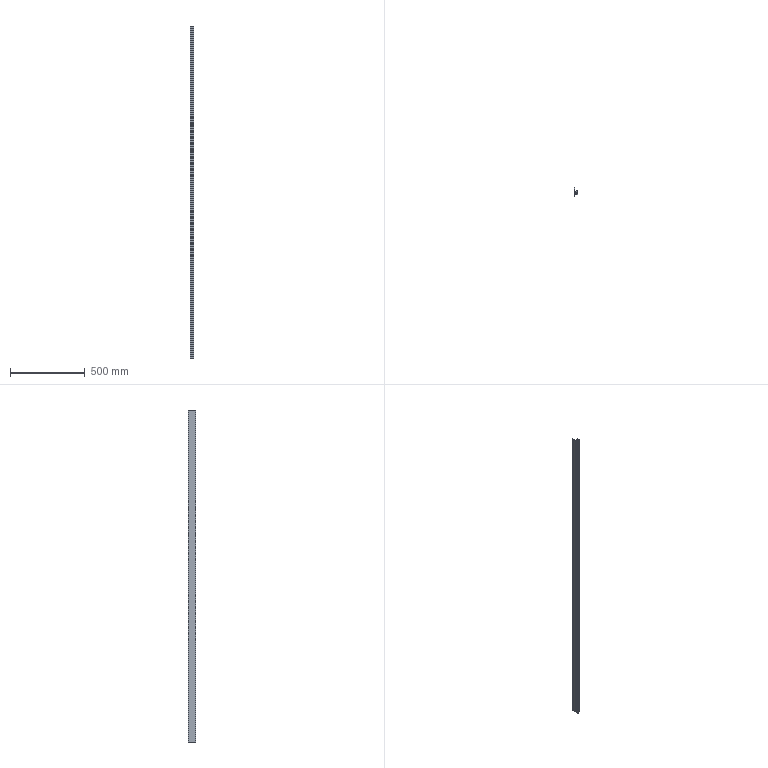Part | SolidWorks | features Extrusion 1 | 1 solid | 43 faces | box 25 x 50 x 2216 mm | volume 690351 mm3 | plane 35 | cylinder 8 | commonest cylinder face diameters 0.6 x8
STEP:
#1=CARTESIAN_POINT('',(1.5,0.,1108.));
#2=VERTEX_POINT('',#1);
#3=CARTESIAN_POINT('',(1.5,10.,1108.));
#4=VERTEX_POINT('',#3);
#5=CARTESIAN_POINT('',(1.5,0.,1108.));
#6=DIRECTION('',(0.,1.,0.));
#7=VECTOR('',#6,1000.);
#8=LINE('',#5,#7);
#9=EDGE_CURVE('',#2,#4,#8,.T.);
#10=ORIENTED_EDGE('',*,*,#9,.T.);
#11=CARTESIAN_POINT('',(4.,10.,1108.));
#12=VERTEX_POINT('',#11);
#13=CARTESIAN_POINT('',(1.5,10.,1108.));
#14=DIRECTION('',(1.,0.,0.));
#15=VECTOR('',#14,1000.);
#16=LINE('',#13,#15);
#17=EDGE_CURVE('',#4,#12,#16,.T.);
#18=ORIENTED_EDGE('',*,*,#17,.T.);
#19=CARTESIAN_POINT('',(4.,10.5,1108.));
#20=VERTEX_POINT('',#19);
#21=CARTESIAN_POINT('',(4.,10.,1108.));
#22=DIRECTION('',(0.,1.,0.));
#23=VECTOR('',#22,1000.);
#24=LINE('',#21,#23);
#25=EDGE_CURVE('',#12,#20,#24,.T.);
#26=ORIENTED_EDGE('',*,*,#25,.T.);
#27=CARTESIAN_POINT('',(8.9,10.5,1108.));
#28=VERTEX_POINT('',#27);
#29=CARTESIAN_POINT('',(4.,10.5,1108.));
#30=DIRECTION('',(1.,0.,0.));
#31=VECTOR('',#30,1000.);
#32=LINE('',#29,#31);
#33=EDGE_CURVE('',#20,#28,#32,.T.);
#34=ORIENTED_EDGE('',*,*,#33,.T.);
#35=CARTESIAN_POINT('',(8.9,12.2,1108.));
#36=VERTEX_POINT('',#35);
#37=CARTESIAN_POINT('',(8.9,10.5,1108.));
#38=DIRECTION('',(0.,1.,0.));
#39=VECTOR('',#38,1000.);
#40=LINE('',#37,#39);
#41=EDGE_CURVE('',#28,#36,#40,.T.);
#42=ORIENTED_EDGE('',*,*,#41,.T.);
#43=CARTESIAN_POINT('',(8.6,12.5,1108.));
#44=VERTEX_POINT('',#43);
#45=CARTESIAN_POINT('',(8.6,12.2,1108.));
#46=DIRECTION('',(0.,0.,1.));
#47=DIRECTION('',(1.,0.,0.));
#48=AXIS2_PLACEMENT_3D('',#45,#46,#47);
#49=CIRCLE('',#48,0.3);
#50=EDGE_CURVE('',#36,#44,#49,.T.);
#51=ORIENTED_EDGE('',*,*,#50,.T.);
#52=CARTESIAN_POINT('',(5.05,12.5,1108.));
#53=VERTEX_POINT('',#52);
#54=CARTESIAN_POINT('',(8.6,12.5,1108.));
#55=DIRECTION('',(-1.,0.,0.));
#56=VECTOR('',#55,1000.);
#57=LINE('',#54,#56);
#58=EDGE_CURVE('',#44,#53,#57,.T.);
#59=ORIENTED_EDGE('',*,*,#58,.T.);
#60=CARTESIAN_POINT('',(4.75,12.8,1108.));
#61=VERTEX_POINT('',#60);
#62=CARTESIAN_POINT('',(5.05,12.8,1108.));
#63=DIRECTION('',(0.,0.,-1.));
#64=DIRECTION('',(1.,0.,0.));
#65=AXIS2_PLACEMENT_3D('',#62,#63,#64);
#66=CIRCLE('',#65,0.3);
#67=EDGE_CURVE('',#53,#61,#66,.T.);
#68=ORIENTED_EDGE('',*,*,#67,.T.);
#69=CARTESIAN_POINT('',(4.75,16.153,1108.));
#70=VERTEX_POINT('',#69);
#71=CARTESIAN_POINT('',(4.75,12.8,1108.));
#72=DIRECTION('',(0.,1.,0.));
#73=VECTOR('',#72,1000.);
#74=LINE('',#71,#73);
#75=EDGE_CURVE('',#61,#70,#74,.T.);
#76=ORIENTED_EDGE('',*,*,#75,.T.);
#77=CARTESIAN_POINT('',(4.838,16.365,1108.));
#78=VERTEX_POINT('',#77);
#79=CARTESIAN_POINT('',(5.05,16.153,1108.));
#80=DIRECTION('',(0.,0.,-1.));
#81=DIRECTION('',(1.,0.,0.));
#82=AXIS2_PLACEMENT_3D('',#79,#80,#81);
#83=CIRCLE('',#82,0.3);
#84=EDGE_CURVE('',#70,#78,#83,.T.);
#85=ORIENTED_EDGE('',*,*,#84,.T.);
#86=CARTESIAN_POINT('',(8.785,20.312,1108.));
#87=VERTEX_POINT('',#86);
#88=CARTESIAN_POINT('',(4.838,16.365,1108.));
#89=DIRECTION('',(0.7071,0.7071,0.));
#90=VECTOR('',#89,1000.);
#91=LINE('',#88,#90);
#92=EDGE_CURVE('',#78,#87,#91,.T.);
#93=ORIENTED_EDGE('',*,*,#92,.T.);
#94=CARTESIAN_POINT('',(8.997,20.4,1108.));
#95=VERTEX_POINT('',#94);
#96=CARTESIAN_POINT('',(8.997,20.1,1108.));
#97=DIRECTION('',(0.,0.,-1.));
#98=DIRECTION('',(1.,0.,0.));
#99=AXIS2_PLACEMENT_3D('',#96,#97,#98);
#100=CIRCLE('',#99,0.3);
#101=EDGE_CURVE('',#87,#95,#100,.T.);
#102=ORIENTED_EDGE('',*,*,#101,.T.);
#103=CARTESIAN_POINT('',(17.003,20.4,1108.));
#104=VERTEX_POINT('',#103);
#105=CARTESIAN_POINT('',(8.997,20.4,1108.));
#106=DIRECTION('',(1.,0.,0.));
#107=VECTOR('',#106,1000.);
#108=LINE('',#105,#107);
#109=EDGE_CURVE('',#95,#104,#108,.T.);
#110=ORIENTED_EDGE('',*,*,#109,.T.);
#111=CARTESIAN_POINT('',(17.215,20.312,1108.));
#112=VERTEX_POINT('',#111);
#113=CARTESIAN_POINT('',(17.003,20.1,1108.));
#114=DIRECTION('',(0.,0.,-1.));
#115=DIRECTION('',(1.,0.,0.));
#116=AXIS2_PLACEMENT_3D('',#113,#114,#115);
#117=CIRCLE('',#116,0.3);
#118=EDGE_CURVE('',#104,#112,#117,.T.);
#119=ORIENTED_EDGE('',*,*,#118,.T.);
#120=CARTESIAN_POINT('',(21.162,16.365,1108.));
#121=VERTEX_POINT('',#120);
#122=CARTESIAN_POINT('',(17.215,20.312,1108.));
#123=DIRECTION('',(0.7071,-0.7071,0.));
#124=VECTOR('',#123,1000.);
#125=LINE('',#122,#124);
#126=EDGE_CURVE('',#112,#121,#125,.T.);
#127=ORIENTED_EDGE('',*,*,#126,.T.);
#128=CARTESIAN_POINT('',(21.25,16.153,1108.));
#129=VERTEX_POINT('',#128);
#130=CARTESIAN_POINT('',(20.95,16.153,1108.));
#131=DIRECTION('',(0.,0.,-1.));
#132=DIRECTION('',(1.,0.,0.));
#133=AXIS2_PLACEMENT_3D('',#130,#131,#132);
#134=CIRCLE('',#133,0.3);
#135=EDGE_CURVE('',#121,#129,#134,.T.);
#136=ORIENTED_EDGE('',*,*,#135,.T.);
#137=CARTESIAN_POINT('',(21.25,12.8,1108.));
#138=VERTEX_POINT('',#137);
#139=CARTESIAN_POINT('',(21.25,16.153,1108.));
#140=DIRECTION('',(0.,-1.,0.));
#141=VECTOR('',#140,1000.);
#142=LINE('',#139,#141);
#143=EDGE_CURVE('',#129,#138,#142,.T.);
#144=ORIENTED_EDGE('',*,*,#143,.T.);
#145=CARTESIAN_POINT('',(20.95,12.5,1108.));
#146=VERTEX_POINT('',#145);
#147=CARTESIAN_POINT('',(20.95,12.8,1108.));
#148=DIRECTION('',(0.,0.,-1.));
#149=DIRECTION('',(1.,0.,0.));
#150=AXIS2_PLACEMENT_3D('',#147,#148,#149);
#151=CIRCLE('',#150,0.3);
#152=EDGE_CURVE('',#138,#146,#151,.T.);
#153=ORIENTED_EDGE('',*,*,#152,.T.);
#154=CARTESIAN_POINT('',(17.4,12.5,1108.));
#155=VERTEX_POINT('',#154);
#156=CARTESIAN_POINT('',(20.95,12.5,1108.));
#157=DIRECTION('',(-1.,0.,0.));
#158=VECTOR('',#157,1000.);
#159=LINE('',#156,#158);
#160=EDGE_CURVE('',#146,#155,#159,.T.);
#161=ORIENTED_EDGE('',*,*,#160,.T.);
#162=CARTESIAN_POINT('',(17.1,12.2,1108.));
#163=VERTEX_POINT('',#162);
#164=CARTESIAN_POINT('',(17.4,12.2,1108.));
#165=DIRECTION('',(0.,0.,1.));
#166=DIRECTION('',(1.,0.,0.));
#167=AXIS2_PLACEMENT_3D('',#164,#165,#166);
#168=CIRCLE('',#167,0.3);
#169=EDGE_CURVE('',#155,#163,#168,.T.);
#170=ORIENTED_EDGE('',*,*,#169,.T.);
#171=CARTESIAN_POINT('',(17.1,10.5,1108.));
#172=VERTEX_POINT('',#171);
#173=CARTESIAN_POINT('',(17.1,12.2,1108.));
#174=DIRECTION('',(0.,-1.,0.));
#175=VECTOR('',#174,1000.);
#176=LINE('',#173,#175);
#177=EDGE_CURVE('',#163,#172,#176,.T.);
#178=ORIENTED_EDGE('',*,*,#177,.T.);
#179=CARTESIAN_POINT('',(22.,10.5,1108.));
#180=VERTEX_POINT('',#179);
#181=CARTESIAN_POINT('',(17.1,10.5,1108.));
#182=DIRECTION('',(1.,0.,0.));
#183=VECTOR('',#182,1000.);
#184=LINE('',#181,#183);
#185=EDGE_CURVE('',#172,#180,#184,.T.);
#186=ORIENTED_EDGE('',*,*,#185,.T.);
#187=CARTESIAN_POINT('',(22.,10.,1108.));
#188=VERTEX_POINT('',#187);
#189=CARTESIAN_POINT('',(22.,10.5,1108.));
#190=DIRECTION('',(0.,-1.,0.));
#191=VECTOR('',#190,1000.);
#192=LINE('',#189,#191);
#193=EDGE_CURVE('',#180,#188,#192,.T.);
#194=ORIENTED_EDGE('',*,*,#193,.T.);
#195=CARTESIAN_POINT('',(25.,10.,1108.));
#196=VERTEX_POINT('',#195);
#197=CARTESIAN_POINT('',(22.,10.,1108.));
#198=DIRECTION('',(1.,0.,0.));
#199=VECTOR('',#198,1000.);
#200=LINE('',#197,#199);
#201=EDGE_CURVE('',#188,#196,#200,.T.);
#202=ORIENTED_EDGE('',*,*,#201,.T.);
#203=CARTESIAN_POINT('',(25.,15.,1108.));
#204=VERTEX_POINT('',#203);
#205=CARTESIAN_POINT('',(25.,10.,1108.));
#206=DIRECTION('',(0.,1.,0.));
#207=VECTOR('',#206,1000.);
#208=LINE('',#205,#207);
#209=EDGE_CURVE('',#196,#204,#208,.T.);
#210=ORIENTED_EDGE('',*,*,#209,.T.);
#211=CARTESIAN_POINT('',(23.,15.,1108.));
#212=VERTEX_POINT('',#211);
#213=CARTESIAN_POINT('',(25.,15.,1108.));
#214=DIRECTION('',(-1.,0.,0.));
#215=VECTOR('',#214,1000.);
#216=LINE('',#213,#215);
#217=EDGE_CURVE('',#204,#212,#216,.T.);
#218=ORIENTED_EDGE('',*,*,#217,.T.);
#219=CARTESIAN_POINT('',(23.,29.246,1108.));
#220=VERTEX_POINT('',#219);
#221=CARTESIAN_POINT('',(23.,15.,1108.));
#222=DIRECTION('',(0.,1.,0.));
#223=VECTOR('',#222,1000.);
#224=LINE('',#221,#223);
#225=EDGE_CURVE('',#212,#220,#224,.T.);
#226=ORIENTED_EDGE('',*,*,#225,.T.);
#227=CARTESIAN_POINT('',(22.25,29.996,1108.));
#228=VERTEX_POINT('',#227);
#229=CARTESIAN_POINT('',(23.,29.246,1108.));
#230=DIRECTION('',(-0.7071,0.7071,0.));
#231=VECTOR('',#230,1000.);
#232=LINE('',#229,#231);
#233=EDGE_CURVE('',#220,#228,#232,.T.);
#234=ORIENTED_EDGE('',*,*,#233,.T.);
#235=CARTESIAN_POINT('',(4.,30.,1108.));
#236=VERTEX_POINT('',#235);
#237=CARTESIAN_POINT('',(22.25,29.996,1108.));
#238=DIRECTION('',(-1.,0.0002341,0.));
#239=VECTOR('',#238,1000.);
#240=LINE('',#237,#239);
#241=EDGE_CURVE('',#228,#236,#240,.T.);
#242=ORIENTED_EDGE('',*,*,#241,.T.);
#243=CARTESIAN_POINT('',(4.,34.998,1108.));
#244=VERTEX_POINT('',#243);
#245=CARTESIAN_POINT('',(4.,30.,1108.));
#246=DIRECTION('',(0.,1.,0.));
#247=VECTOR('',#246,1000.);
#248=LINE('',#245,#247);
#249=EDGE_CURVE('',#236,#244,#248,.T.);
#250=ORIENTED_EDGE('',*,*,#249,.T.);
#251=CARTESIAN_POINT('',(3.,34.998,1108.));
#252=VERTEX_POINT('',#251);
#253=CARTESIAN_POINT('',(4.,34.998,1108.));
#254=DIRECTION('',(-1.,0.,0.));
#255=VECTOR('',#254,1000.);
#256=LINE('',#253,#255);
#257=EDGE_CURVE('',#244,#252,#256,.T.);
#258=ORIENTED_EDGE('',*,*,#257,.T.);
#259=CARTESIAN_POINT('',(3.,43.,1108.));
#260=VERTEX_POINT('',#259);
#261=CARTESIAN_POINT('',(3.,34.998,1108.));
#262=DIRECTION('',(0.,1.,0.));
#263=VECTOR('',#262,1000.);
#264=LINE('',#261,#263);
#265=EDGE_CURVE('',#252,#260,#264,.T.);
#266=ORIENTED_EDGE('',*,*,#265,.T.);
#267=CARTESIAN_POINT('',(4.,43.,1108.));
#268=VERTEX_POINT('',#267);
#269=CARTESIAN_POINT('',(3.,43.,1108.));
#270=DIRECTION('',(1.,0.,0.));
#271=VECTOR('',#270,1000.);
#272=LINE('',#269,#271);
#273=EDGE_CURVE('',#260,#268,#272,.T.);
#274=ORIENTED_EDGE('',*,*,#273,.T.);
#275=CARTESIAN_POINT('',(4.,50.,1108.));
#276=VERTEX_POINT('',#275);
#277=CARTESIAN_POINT('',(4.,43.,1108.));
#278=DIRECTION('',(0.,1.,0.));
#279=VECTOR('',#278,1000.);
#280=LINE('',#277,#279);
#281=EDGE_CURVE('',#268,#276,#280,.T.);
#282=ORIENTED_EDGE('',*,*,#281,.T.);
#283=CARTESIAN_POINT('',(0.,50.,1108.));
#284=VERTEX_POINT('',#283);
#285=CARTESIAN_POINT('',(4.,50.,1108.));
#286=DIRECTION('',(-1.,0.,0.));
#287=VECTOR('',#286,1000.);
#288=LINE('',#285,#287);
#289=EDGE_CURVE('',#276,#284,#288,.T.);
#290=ORIENTED_EDGE('',*,*,#289,.T.);
#291=CARTESIAN_POINT('',(0.,0.,1108.));
#292=VERTEX_POINT('',#291);
#293=CARTESIAN_POINT('',(0.,50.,1108.));
#294=DIRECTION('',(0.,-1.,0.));
#295=VECTOR('',#294,1000.);
#296=LINE('',#293,#295);
#297=EDGE_CURVE('',#284,#292,#296,.T.);
#298=ORIENTED_EDGE('',*,*,#297,.T.);
#299=CARTESIAN_POINT('',(0.,0.,1108.));
#300=DIRECTION('',(1.,0.,0.));
#301=VECTOR('',#300,1000.);
#302=LINE('',#299,#301);
#303=EDGE_CURVE('',#292,#2,#302,.T.);
#304=ORIENTED_EDGE('',*,*,#303,.T.);
#305=EDGE_LOOP('',(#10,#18,#26,#34,#42,#51,#59,#68,#76,#85,#93,#102,#110,#119,#127,#136,#144,#153,#161,#170,#178,#186,#194,#202,#210,#218,#226,#234,#242,#250,#258,#266,#274,#282,#290,#298,#304));
#306=FACE_OUTER_BOUND('',#305,.T.);
#307=CARTESIAN_POINT('',(21.,28.,1108.));
#308=VERTEX_POINT('',#307);
#309=CARTESIAN_POINT('',(2.,28.,1108.));
#310=VERTEX_POINT('',#309);
#311=CARTESIAN_POINT('',(2.,28.,1108.));
#312=DIRECTION('',(-1.,0.,0.));
#313=VECTOR('',#312,1000.);
#314=LINE('',#311,#313);
#315=EDGE_CURVE('',#308,#310,#314,.T.);
#316=ORIENTED_EDGE('',*,*,#315,.F.);
#317=CARTESIAN_POINT('',(21.,22.4,1108.));
#318=VERTEX_POINT('',#317);
#319=CARTESIAN_POINT('',(21.,28.,1108.));
#320=DIRECTION('',(0.,1.,0.));
#321=VECTOR('',#320,1000.);
#322=LINE('',#319,#321);
#323=EDGE_CURVE('',#318,#308,#322,.T.);
#324=ORIENTED_EDGE('',*,*,#323,.F.);
#325=CARTESIAN_POINT('',(2.,22.4,1108.));
#326=VERTEX_POINT('',#325);
#327=CARTESIAN_POINT('',(21.,22.4,1108.));
#328=DIRECTION('',(1.,0.,0.));
#329=VECTOR('',#328,1000.);
#330=LINE('',#327,#329);
#331=EDGE_CURVE('',#326,#318,#330,.T.);
#332=ORIENTED_EDGE('',*,*,#331,.F.);
#333=CARTESIAN_POINT('',(2.,22.4,1108.));
#334=DIRECTION('',(0.,-1.,0.));
#335=VECTOR('',#334,1000.);
#336=LINE('',#333,#335);
#337=EDGE_CURVE('',#310,#326,#336,.T.);
#338=ORIENTED_EDGE('',*,*,#337,.F.);
#339=EDGE_LOOP('',(#316,#324,#332,#338));
#340=FACE_BOUND('',#339,.T.);
#341=CARTESIAN_POINT('',(8.6,12.2,1108.));
#342=DIRECTION('',(0.,0.,1.));
#343=DIRECTION('',(1.,0.,0.));
#344=AXIS2_PLACEMENT_3D('',#341,#342,#343);
#345=PLANE('',#344);
#346=ADVANCED_FACE('',(#306,#340),#345,.T.);
#347=CARTESIAN_POINT('',(1.5,0.,-1108.));
#348=VERTEX_POINT('',#347);
#349=CARTESIAN_POINT('',(1.5,10.,-1108.));
#350=VERTEX_POINT('',#349);
#351=CARTESIAN_POINT('',(1.5,0.,-1108.));
#352=DIRECTION('',(0.,1.,0.));
#353=VECTOR('',#352,1000.);
#354=LINE('',#351,#353);
#355=EDGE_CURVE('',#348,#350,#354,.T.);
#356=ORIENTED_EDGE('',*,*,#355,.F.);
#357=CARTESIAN_POINT('',(0.,0.,-1108.));
#358=VERTEX_POINT('',#357);
#359=CARTESIAN_POINT('',(0.,0.,-1108.));
#360=DIRECTION('',(1.,0.,0.));
#361=VECTOR('',#360,1000.);
#362=LINE('',#359,#361);
#363=EDGE_CURVE('',#358,#348,#362,.T.);
#364=ORIENTED_EDGE('',*,*,#363,.F.);
#365=CARTESIAN_POINT('',(0.,50.,-1108.));
#366=VERTEX_POINT('',#365);
#367=CARTESIAN_POINT('',(0.,50.,-1108.));
#368=DIRECTION('',(0.,-1.,0.));
#369=VECTOR('',#368,1000.);
#370=LINE('',#367,#369);
#371=EDGE_CURVE('',#366,#358,#370,.T.);
#372=ORIENTED_EDGE('',*,*,#371,.F.);
#373=CARTESIAN_POINT('',(4.,50.,-1108.));
#374=VERTEX_POINT('',#373);
#375=CARTESIAN_POINT('',(4.,50.,-1108.));
#376=DIRECTION('',(-1.,0.,0.));
#377=VECTOR('',#376,1000.);
#378=LINE('',#375,#377);
#379=EDGE_CURVE('',#374,#366,#378,.T.);
#380=ORIENTED_EDGE('',*,*,#379,.F.);
#381=CARTESIAN_POINT('',(4.,43.,-1108.));
#382=VERTEX_POINT('',#381);
#383=CARTESIAN_POINT('',(4.,43.,-1108.));
#384=DIRECTION('',(0.,1.,0.));
#385=VECTOR('',#384,1000.);
#386=LINE('',#383,#385);
#387=EDGE_CURVE('',#382,#374,#386,.T.);
#388=ORIENTED_EDGE('',*,*,#387,.F.);
#389=CARTESIAN_POINT('',(3.,43.,-1108.));
#390=VERTEX_POINT('',#389);
#391=CARTESIAN_POINT('',(3.,43.,-1108.));
#392=DIRECTION('',(1.,0.,0.));
#393=VECTOR('',#392,1000.);
#394=LINE('',#391,#393);
#395=EDGE_CURVE('',#390,#382,#394,.T.);
#396=ORIENTED_EDGE('',*,*,#395,.F.);
#397=CARTESIAN_POINT('',(3.,34.998,-1108.));
#398=VERTEX_POINT('',#397);
#399=CARTESIAN_POINT('',(3.,34.998,-1108.));
#400=DIRECTION('',(0.,1.,0.));
#401=VECTOR('',#400,1000.);
#402=LINE('',#399,#401);
#403=EDGE_CURVE('',#398,#390,#402,.T.);
#404=ORIENTED_EDGE('',*,*,#403,.F.);
#405=CARTESIAN_POINT('',(4.,34.998,-1108.));
#406=VERTEX_POINT('',#405);
#407=CARTESIAN_POINT('',(4.,34.998,-1108.));
#408=DIRECTION('',(-1.,0.,0.));
#409=VECTOR('',#408,1000.);
#410=LINE('',#407,#409);
#411=EDGE_CURVE('',#406,#398,#410,.T.);
#412=ORIENTED_EDGE('',*,*,#411,.F.);
#413=CARTESIAN_POINT('',(4.,30.,-1108.));
#414=VERTEX_POINT('',#413);
#415=CARTESIAN_POINT('',(4.,30.,-1108.));
#416=DIRECTION('',(0.,1.,0.));
#417=VECTOR('',#416,1000.);
#418=LINE('',#415,#417);
#419=EDGE_CURVE('',#414,#406,#418,.T.);
#420=ORIENTED_EDGE('',*,*,#419,.F.);
#421=CARTESIAN_POINT('',(22.25,29.996,-1108.));
#422=VERTEX_POINT('',#421);
#423=CARTESIAN_POINT('',(22.25,29.996,-1108.));
#424=DIRECTION('',(-1.,0.0002341,0.));
#425=VECTOR('',#424,1000.);
#426=LINE('',#423,#425);
#427=EDGE_CURVE('',#422,#414,#426,.T.);
#428=ORIENTED_EDGE('',*,*,#427,.F.);
#429=CARTESIAN_POINT('',(23.,29.246,-1108.));
#430=VERTEX_POINT('',#429);
#431=CARTESIAN_POINT('',(23.,29.246,-1108.));
#432=DIRECTION('',(-0.7071,0.7071,0.));
#433=VECTOR('',#432,1000.);
#434=LINE('',#431,#433);
#435=EDGE_CURVE('',#430,#422,#434,.T.);
#436=ORIENTED_EDGE('',*,*,#435,.F.);
#437=CARTESIAN_POINT('',(23.,15.,-1108.));
#438=VERTEX_POINT('',#437);
#439=CARTESIAN_POINT('',(23.,15.,-1108.));
#440=DIRECTION('',(0.,1.,0.));
#441=VECTOR('',#440,1000.);
#442=LINE('',#439,#441);
#443=EDGE_CURVE('',#438,#430,#442,.T.);
#444=ORIENTED_EDGE('',*,*,#443,.F.);
#445=CARTESIAN_POINT('',(25.,15.,-1108.));
#446=VERTEX_POINT('',#445);
#447=CARTESIAN_POINT('',(25.,15.,-1108.));
#448=DIRECTION('',(-1.,0.,0.));
#449=VECTOR('',#448,1000.);
#450=LINE('',#447,#449);
#451=EDGE_CURVE('',#446,#438,#450,.T.);
#452=ORIENTED_EDGE('',*,*,#451,.F.);
#453=CARTESIAN_POINT('',(25.,10.,-1108.));
#454=VERTEX_POINT('',#453);
#455=CARTESIAN_POINT('',(25.,10.,-1108.));
#456=DIRECTION('',(0.,1.,0.));
#457=VECTOR('',#456,1000.);
#458=LINE('',#455,#457);
#459=EDGE_CURVE('',#454,#446,#458,.T.);
#460=ORIENTED_EDGE('',*,*,#459,.F.);
#461=CARTESIAN_POINT('',(22.,10.,-1108.));
#462=VERTEX_POINT('',#461);
#463=CARTESIAN_POINT('',(22.,10.,-1108.));
#464=DIRECTION('',(1.,0.,0.));
#465=VECTOR('',#464,1000.);
#466=LINE('',#463,#465);
#467=EDGE_CURVE('',#462,#454,#466,.T.);
#468=ORIENTED_EDGE('',*,*,#467,.F.);
#469=CARTESIAN_POINT('',(22.,10.5,-1108.));
#470=VERTEX_POINT('',#469);
#471=CARTESIAN_POINT('',(22.,10.5,-1108.));
#472=DIRECTION('',(0.,-1.,0.));
#473=VECTOR('',#472,1000.);
#474=LINE('',#471,#473);
#475=EDGE_CURVE('',#470,#462,#474,.T.);
#476=ORIENTED_EDGE('',*,*,#475,.F.);
#477=CARTESIAN_POINT('',(17.1,10.5,-1108.));
#478=VERTEX_POINT('',#477);
#479=CARTESIAN_POINT('',(17.1,10.5,-1108.));
#480=DIRECTION('',(1.,0.,0.));
#481=VECTOR('',#480,1000.);
#482=LINE('',#479,#481);
#483=EDGE_CURVE('',#478,#470,#482,.T.);
#484=ORIENTED_EDGE('',*,*,#483,.F.);
#485=CARTESIAN_POINT('',(17.1,12.2,-1108.));
#486=VERTEX_POINT('',#485);
#487=CARTESIAN_POINT('',(17.1,12.2,-1108.));
#488=DIRECTION('',(0.,-1.,0.));
#489=VECTOR('',#488,1000.);
#490=LINE('',#487,#489);
#491=EDGE_CURVE('',#486,#478,#490,.T.);
#492=ORIENTED_EDGE('',*,*,#491,.F.);
#493=CARTESIAN_POINT('',(17.4,12.5,-1108.));
#494=VERTEX_POINT('',#493);
#495=CARTESIAN_POINT('',(17.4,12.2,-1108.));
#496=DIRECTION('',(0.,0.,1.));
#497=DIRECTION('',(1.,0.,0.));
#498=AXIS2_PLACEMENT_3D('',#495,#496,#497);
#499=CIRCLE('',#498,0.3);
#500=EDGE_CURVE('',#494,#486,#499,.T.);
#501=ORIENTED_EDGE('',*,*,#500,.F.);
#502=CARTESIAN_POINT('',(20.95,12.5,-1108.));
#503=VERTEX_POINT('',#502);
#504=CARTESIAN_POINT('',(20.95,12.5,-1108.));
#505=DIRECTION('',(-1.,0.,0.));
#506=VECTOR('',#505,1000.);
#507=LINE('',#504,#506);
#508=EDGE_CURVE('',#503,#494,#507,.T.);
#509=ORIENTED_EDGE('',*,*,#508,.F.);
#510=CARTESIAN_POINT('',(21.25,12.8,-1108.));
#511=VERTEX_POINT('',#510);
#512=CARTESIAN_POINT('',(20.95,12.8,-1108.));
#513=DIRECTION('',(0.,0.,-1.));
#514=DIRECTION('',(1.,0.,0.));
#515=AXIS2_PLACEMENT_3D('',#512,#513,#514);
#516=CIRCLE('',#515,0.3);
#517=EDGE_CURVE('',#511,#503,#516,.T.);
#518=ORIENTED_EDGE('',*,*,#517,.F.);
#519=CARTESIAN_POINT('',(21.25,16.153,-1108.));
#520=VERTEX_POINT('',#519);
#521=CARTESIAN_POINT('',(21.25,16.153,-1108.));
#522=DIRECTION('',(0.,-1.,0.));
#523=VECTOR('',#522,1000.);
#524=LINE('',#521,#523);
#525=EDGE_CURVE('',#520,#511,#524,.T.);
#526=ORIENTED_EDGE('',*,*,#525,.F.);
#527=CARTESIAN_POINT('',(21.162,16.365,-1108.));
#528=VERTEX_POINT('',#527);
#529=CARTESIAN_POINT('',(20.95,16.153,-1108.));
#530=DIRECTION('',(0.,0.,-1.));
#531=DIRECTION('',(1.,0.,0.));
#532=AXIS2_PLACEMENT_3D('',#529,#530,#531);
#533=CIRCLE('',#532,0.3);
#534=EDGE_CURVE('',#528,#520,#533,.T.);
#535=ORIENTED_EDGE('',*,*,#534,.F.);
#536=CARTESIAN_POINT('',(17.215,20.312,-1108.));
#537=VERTEX_POINT('',#536);
#538=CARTESIAN_POINT('',(17.215,20.312,-1108.));
#539=DIRECTION('',(0.7071,-0.7071,0.));
#540=VECTOR('',#539,1000.);
#541=LINE('',#538,#540);
#542=EDGE_CURVE('',#537,#528,#541,.T.);
#543=ORIENTED_EDGE('',*,*,#542,.F.);
#544=CARTESIAN_POINT('',(17.003,20.4,-1108.));
#545=VERTEX_POINT('',#544);
#546=CARTESIAN_POINT('',(17.003,20.1,-1108.));
#547=DIRECTION('',(0.,0.,-1.));
#548=DIRECTION('',(1.,0.,0.));
#549=AXIS2_PLACEMENT_3D('',#546,#547,#548);
#550=CIRCLE('',#549,0.3);
#551=EDGE_CURVE('',#545,#537,#550,.T.);
#552=ORIENTED_EDGE('',*,*,#551,.F.);
#553=CARTESIAN_POINT('',(8.997,20.4,-1108.));
#554=VERTEX_POINT('',#553);
#555=CARTESIAN_POINT('',(8.997,20.4,-1108.));
#556=DIRECTION('',(1.,0.,0.));
#557=VECTOR('',#556,1000.);
#558=LINE('',#555,#557);
#559=EDGE_CURVE('',#554,#545,#558,.T.);
#560=ORIENTED_EDGE('',*,*,#559,.F.);
#561=CARTESIAN_POINT('',(8.785,20.312,-1108.));
#562=VERTEX_POINT('',#561);
#563=CARTESIAN_POINT('',(8.997,20.1,-1108.));
#564=DIRECTION('',(0.,0.,-1.));
#565=DIRECTION('',(1.,0.,0.));
#566=AXIS2_PLACEMENT_3D('',#563,#564,#565);
#567=CIRCLE('',#566,0.3);
#568=EDGE_CURVE('',#562,#554,#567,.T.);
#569=ORIENTED_EDGE('',*,*,#568,.F.);
#570=CARTESIAN_POINT('',(4.838,16.365,-1108.));
#571=VERTEX_POINT('',#570);
#572=CARTESIAN_POINT('',(4.838,16.365,-1108.));
#573=DIRECTION('',(0.7071,0.7071,0.));
#574=VECTOR('',#573,1000.);
#575=LINE('',#572,#574);
#576=EDGE_CURVE('',#571,#562,#575,.T.);
#577=ORIENTED_EDGE('',*,*,#576,.F.);
#578=CARTESIAN_POINT('',(4.75,16.153,-1108.));
#579=VERTEX_POINT('',#578);
#580=CARTESIAN_POINT('',(5.05,16.153,-1108.));
#581=DIRECTION('',(0.,0.,-1.));
#582=DIRECTION('',(1.,0.,0.));
#583=AXIS2_PLACEMENT_3D('',#580,#581,#582);
#584=CIRCLE('',#583,0.3);
#585=EDGE_CURVE('',#579,#571,#584,.T.);
#586=ORIENTED_EDGE('',*,*,#585,.F.);
#587=CARTESIAN_POINT('',(4.75,12.8,-1108.));
#588=VERTEX_POINT('',#587);
#589=CARTESIAN_POINT('',(4.75,12.8,-1108.));
#590=DIRECTION('',(0.,1.,0.));
#591=VECTOR('',#590,1000.);
#592=LINE('',#589,#591);
#593=EDGE_CURVE('',#588,#579,#592,.T.);
#594=ORIENTED_EDGE('',*,*,#593,.F.);
#595=CARTESIAN_POINT('',(5.05,12.5,-1108.));
#596=VERTEX_POINT('',#595);
#597=CARTESIAN_POINT('',(5.05,12.8,-1108.));
#598=DIRECTION('',(0.,0.,-1.));
#599=DIRECTION('',(1.,0.,0.));
#600=AXIS2_PLACEMENT_3D('',#597,#598,#599);
#601=CIRCLE('',#600,0.3);
#602=EDGE_CURVE('',#596,#588,#601,.T.);
#603=ORIENTED_EDGE('',*,*,#602,.F.);
#604=CARTESIAN_POINT('',(8.6,12.5,-1108.));
#605=VERTEX_POINT('',#604);
#606=CARTESIAN_POINT('',(8.6,12.5,-1108.));
#607=DIRECTION('',(-1.,0.,0.));
#608=VECTOR('',#607,1000.);
#609=LINE('',#606,#608);
#610=EDGE_CURVE('',#605,#596,#609,.T.);
#611=ORIENTED_EDGE('',*,*,#610,.F.);
#612=CARTESIAN_POINT('',(8.9,12.2,-1108.));
#613=VERTEX_POINT('',#612);
#614=CARTESIAN_POINT('',(8.6,12.2,-1108.));
#615=DIRECTION('',(0.,0.,1.));
#616=DIRECTION('',(1.,0.,0.));
#617=AXIS2_PLACEMENT_3D('',#614,#615,#616);
#618=CIRCLE('',#617,0.3);
#619=EDGE_CURVE('',#613,#605,#618,.T.);
#620=ORIENTED_EDGE('',*,*,#619,.F.);
#621=CARTESIAN_POINT('',(8.9,10.5,-1108.));
#622=VERTEX_POINT('',#621);
#623=CARTESIAN_POINT('',(8.9,10.5,-1108.));
#624=DIRECTION('',(0.,1.,0.));
#625=VECTOR('',#624,1000.);
#626=LINE('',#623,#625);
#627=EDGE_CURVE('',#622,#613,#626,.T.);
#628=ORIENTED_EDGE('',*,*,#627,.F.);
#629=CARTESIAN_POINT('',(4.,10.5,-1108.));
#630=VERTEX_POINT('',#629);
#631=CARTESIAN_POINT('',(4.,10.5,-1108.));
#632=DIRECTION('',(1.,0.,0.));
#633=VECTOR('',#632,1000.);
#634=LINE('',#631,#633);
#635=EDGE_CURVE('',#630,#622,#634,.T.);
#636=ORIENTED_EDGE('',*,*,#635,.F.);
#637=CARTESIAN_POINT('',(4.,10.,-1108.));
#638=VERTEX_POINT('',#637);
#639=CARTESIAN_POINT('',(4.,10.,-1108.));
#640=DIRECTION('',(0.,1.,0.));
#641=VECTOR('',#640,1000.);
#642=LINE('',#639,#641);
#643=EDGE_CURVE('',#638,#630,#642,.T.);
#644=ORIENTED_EDGE('',*,*,#643,.F.);
#645=CARTESIAN_POINT('',(1.5,10.,-1108.));
#646=DIRECTION('',(1.,0.,0.));
#647=VECTOR('',#646,1000.);
#648=LINE('',#645,#647);
#649=EDGE_CURVE('',#350,#638,#648,.T.);
#650=ORIENTED_EDGE('',*,*,#649,.F.);
#651=EDGE_LOOP('',(#356,#364,#372,#380,#388,#396,#404,#412,#420,#428,#436,#444,#452,#460,#468,#476,#484,#492,#501,#509,#518,#526,#535,#543,#552,#560,#569,#577,#586,#594,#603,#611,#620,#628,#636,#644,#650));
#652=FACE_OUTER_BOUND('',#651,.T.);
#653=CARTESIAN_POINT('',(21.,22.4,-1108.));
#654=VERTEX_POINT('',#653);
#655=CARTESIAN_POINT('',(21.,28.,-1108.));
#656=VERTEX_POINT('',#655);
#657=CARTESIAN_POINT('',(21.,28.,-1108.));
#658=DIRECTION('',(0.,1.,0.));
#659=VECTOR('',#658,1000.);
#660=LINE('',#657,#659);
#661=EDGE_CURVE('',#654,#656,#660,.T.);
#662=ORIENTED_EDGE('',*,*,#661,.T.);
#663=CARTESIAN_POINT('',(2.,28.,-1108.));
#664=VERTEX_POINT('',#663);
#665=CARTESIAN_POINT('',(2.,28.,-1108.));
#666=DIRECTION('',(-1.,0.,0.));
#667=VECTOR('',#666,1000.);
#668=LINE('',#665,#667);
#669=EDGE_CURVE('',#656,#664,#668,.T.);
#670=ORIENTED_EDGE('',*,*,#669,.T.);
#671=CARTESIAN_POINT('',(2.,22.4,-1108.));
#672=VERTEX_POINT('',#671);
#673=CARTESIAN_POINT('',(2.,22.4,-1108.));
#674=DIRECTION('',(0.,-1.,0.));
#675=VECTOR('',#674,1000.);
#676=LINE('',#673,#675);
#677=EDGE_CURVE('',#664,#672,#676,.T.);
#678=ORIENTED_EDGE('',*,*,#677,.T.);
#679=CARTESIAN_POINT('',(21.,22.4,-1108.));
#680=DIRECTION('',(1.,0.,0.));
#681=VECTOR('',#680,1000.);
#682=LINE('',#679,#681);
#683=EDGE_CURVE('',#672,#654,#682,.T.);
#684=ORIENTED_EDGE('',*,*,#683,.T.);
#685=EDGE_LOOP('',(#662,#670,#678,#684));
#686=FACE_BOUND('',#685,.T.);
#687=CARTESIAN_POINT('',(8.6,12.2,-1108.));
#688=DIRECTION('',(0.,0.,1.));
#689=DIRECTION('',(1.,0.,0.));
#690=AXIS2_PLACEMENT_3D('',#687,#688,#689);
#691=PLANE('',#690);
#692=ADVANCED_FACE('',(#652,#686),#691,.F.);
#693=ORIENTED_EDGE('',*,*,#355,.T.);
#694=CARTESIAN_POINT('',(1.5,10.,1108.));
#695=DIRECTION('',(0.,0.,-1.));
#696=VECTOR('',#695,1000.);
#697=LINE('',#694,#696);
#698=EDGE_CURVE('',#4,#350,#697,.T.);
#699=ORIENTED_EDGE('',*,*,#698,.F.);
#700=ORIENTED_EDGE('',*,*,#9,.F.);
#701=CARTESIAN_POINT('',(1.5,0.,1108.));
#702=DIRECTION('',(0.,0.,-1.));
#703=VECTOR('',#702,1000.);
#704=LINE('',#701,#703);
#705=EDGE_CURVE('',#2,#348,#704,.T.);
#706=ORIENTED_EDGE('',*,*,#705,.T.);
#707=EDGE_LOOP('',(#693,#699,#700,#706));
#708=FACE_OUTER_BOUND('',#707,.T.);
#709=CARTESIAN_POINT('',(1.5,0.,1108.));
#710=DIRECTION('',(-1.,0.,0.));
#711=DIRECTION('',(0.,0.,1.));
#712=AXIS2_PLACEMENT_3D('',#709,#710,#711);
#713=PLANE('',#712);
#714=ADVANCED_FACE('',(#708),#713,.F.);
#715=ORIENTED_EDGE('',*,*,#649,.T.);
#716=CARTESIAN_POINT('',(4.,10.,1108.));
#717=DIRECTION('',(0.,0.,-1.));
#718=VECTOR('',#717,1000.);
#719=LINE('',#716,#718);
#720=EDGE_CURVE('',#12,#638,#719,.T.);
#721=ORIENTED_EDGE('',*,*,#720,.F.);
#722=ORIENTED_EDGE('',*,*,#17,.F.);
#723=ORIENTED_EDGE('',*,*,#698,.T.);
#724=EDGE_LOOP('',(#715,#721,#722,#723));
#725=FACE_OUTER_BOUND('',#724,.T.);
#726=CARTESIAN_POINT('',(1.5,10.,1108.));
#727=DIRECTION('',(0.,1.,0.));
#728=DIRECTION('',(0.,0.,1.));
#729=AXIS2_PLACEMENT_3D('',#726,#727,#728);
#730=PLANE('',#729);
#731=ADVANCED_FACE('',(#725),#730,.F.);
#732=ORIENTED_EDGE('',*,*,#643,.T.);
#733=CARTESIAN_POINT('',(4.,10.5,1108.));
#734=DIRECTION('',(0.,0.,-1.));
#735=VECTOR('',#734,1000.);
#736=LINE('',#733,#735);
#737=EDGE_CURVE('',#20,#630,#736,.T.);
#738=ORIENTED_EDGE('',*,*,#737,.F.);
#739=ORIENTED_EDGE('',*,*,#25,.F.);
#740=ORIENTED_EDGE('',*,*,#720,.T.);
#741=EDGE_LOOP('',(#732,#738,#739,#740));
#742=FACE_OUTER_BOUND('',#741,.T.);
#743=CARTESIAN_POINT('',(4.,10.,1108.));
#744=DIRECTION('',(-1.,0.,0.));
#745=DIRECTION('',(0.,0.,1.));
#746=AXIS2_PLACEMENT_3D('',#743,#744,#745);
#747=PLANE('',#746);
#748=ADVANCED_FACE('',(#742),#747,.F.);
#749=ORIENTED_EDGE('',*,*,#635,.T.);
#750=CARTESIAN_POINT('',(8.9,10.5,1108.));
#751=DIRECTION('',(0.,0.,-1.));
#752=VECTOR('',#751,1000.);
#753=LINE('',#750,#752);
#754=EDGE_CURVE('',#28,#622,#753,.T.);
#755=ORIENTED_EDGE('',*,*,#754,.F.);
#756=ORIENTED_EDGE('',*,*,#33,.F.);
#757=ORIENTED_EDGE('',*,*,#737,.T.);
#758=EDGE_LOOP('',(#749,#755,#756,#757));
#759=FACE_OUTER_BOUND('',#758,.T.);
#760=CARTESIAN_POINT('',(4.,10.5,1108.));
#761=DIRECTION('',(0.,1.,0.));
#762=DIRECTION('',(0.,0.,1.));
#763=AXIS2_PLACEMENT_3D('',#760,#761,#762);
#764=PLANE('',#763);
#765=ADVANCED_FACE('',(#759),#764,.F.);
#766=ORIENTED_EDGE('',*,*,#627,.T.);
#767=CARTESIAN_POINT('',(8.9,12.2,1108.));
#768=DIRECTION('',(0.,0.,-1.));
#769=VECTOR('',#768,1000.);
#770=LINE('',#767,#769);
#771=EDGE_CURVE('',#36,#613,#770,.T.);
#772=ORIENTED_EDGE('',*,*,#771,.F.);
#773=ORIENTED_EDGE('',*,*,#41,.F.);
#774=ORIENTED_EDGE('',*,*,#754,.T.);
#775=EDGE_LOOP('',(#766,#772,#773,#774));
#776=FACE_OUTER_BOUND('',#775,.T.);
#777=CARTESIAN_POINT('',(8.9,10.5,1108.));
#778=DIRECTION('',(-1.,0.,0.));
#779=DIRECTION('',(0.,0.,1.));
#780=AXIS2_PLACEMENT_3D('',#777,#778,#779);
#781=PLANE('',#780);
#782=ADVANCED_FACE('',(#776),#781,.F.);
#783=ORIENTED_EDGE('',*,*,#619,.T.);
#784=CARTESIAN_POINT('',(8.6,12.5,1108.));
#785=DIRECTION('',(0.,0.,-1.));
#786=VECTOR('',#785,1000.);
#787=LINE('',#784,#786);
#788=EDGE_CURVE('',#44,#605,#787,.T.);
#789=ORIENTED_EDGE('',*,*,#788,.F.);
#790=ORIENTED_EDGE('',*,*,#50,.F.);
#791=ORIENTED_EDGE('',*,*,#771,.T.);
#792=EDGE_LOOP('',(#783,#789,#790,#791));
#793=FACE_OUTER_BOUND('',#792,.T.);
#794=CARTESIAN_POINT('',(8.6,12.2,1108.));
#795=DIRECTION('',(0.,0.,-1.));
#796=DIRECTION('',(-1.,0.,0.));
#797=AXIS2_PLACEMENT_3D('',#794,#795,#796);
#798=CYLINDRICAL_SURFACE('',#797,0.3);
#799=ADVANCED_FACE('',(#793),#798,.T.);
#800=ORIENTED_EDGE('',*,*,#610,.T.);
#801=CARTESIAN_POINT('',(5.05,12.5,1108.));
#802=DIRECTION('',(0.,0.,-1.));
#803=VECTOR('',#802,1000.);
#804=LINE('',#801,#803);
#805=EDGE_CURVE('',#53,#596,#804,.T.);
#806=ORIENTED_EDGE('',*,*,#805,.F.);
#807=ORIENTED_EDGE('',*,*,#58,.F.);
#808=ORIENTED_EDGE('',*,*,#788,.T.);
#809=EDGE_LOOP('',(#800,#806,#807,#808));
#810=FACE_OUTER_BOUND('',#809,.T.);
#811=CARTESIAN_POINT('',(8.6,12.5,1108.));
#812=DIRECTION('',(0.,-1.,0.));
#813=DIRECTION('',(0.,0.,-1.));
#814=AXIS2_PLACEMENT_3D('',#811,#812,#813);
#815=PLANE('',#814);
#816=ADVANCED_FACE('',(#810),#815,.F.);
#817=ORIENTED_EDGE('',*,*,#602,.T.);
#818=CARTESIAN_POINT('',(4.75,12.8,1108.));
#819=DIRECTION('',(0.,0.,-1.));
#820=VECTOR('',#819,1000.);
#821=LINE('',#818,#820);
#822=EDGE_CURVE('',#61,#588,#821,.T.);
#823=ORIENTED_EDGE('',*,*,#822,.F.);
#824=ORIENTED_EDGE('',*,*,#67,.F.);
#825=ORIENTED_EDGE('',*,*,#805,.T.);
#826=EDGE_LOOP('',(#817,#823,#824,#825));
#827=FACE_OUTER_BOUND('',#826,.T.);
#828=CARTESIAN_POINT('',(5.05,12.8,1108.));
#829=DIRECTION('',(0.,0.,-1.));
#830=DIRECTION('',(-1.,0.,0.));
#831=AXIS2_PLACEMENT_3D('',#828,#829,#830);
#832=CYLINDRICAL_SURFACE('',#831,0.3);
#833=ADVANCED_FACE('',(#827),#832,.F.);
#834=ORIENTED_EDGE('',*,*,#593,.T.);
#835=CARTESIAN_POINT('',(4.75,16.153,1108.));
#836=DIRECTION('',(0.,0.,-1.));
#837=VECTOR('',#836,1000.);
#838=LINE('',#835,#837);
#839=EDGE_CURVE('',#70,#579,#838,.T.);
#840=ORIENTED_EDGE('',*,*,#839,.F.);
#841=ORIENTED_EDGE('',*,*,#75,.F.);
#842=ORIENTED_EDGE('',*,*,#822,.T.);
#843=EDGE_LOOP('',(#834,#840,#841,#842));
#844=FACE_OUTER_BOUND('',#843,.T.);
#845=CARTESIAN_POINT('',(4.75,12.8,1108.));
#846=DIRECTION('',(-1.,0.,0.));
#847=DIRECTION('',(0.,0.,1.));
#848=AXIS2_PLACEMENT_3D('',#845,#846,#847);
#849=PLANE('',#848);
#850=ADVANCED_FACE('',(#844),#849,.F.);
#851=ORIENTED_EDGE('',*,*,#585,.T.);
#852=CARTESIAN_POINT('',(4.838,16.365,1108.));
#853=DIRECTION('',(0.,0.,-1.));
#854=VECTOR('',#853,1000.);
#855=LINE('',#852,#854);
#856=EDGE_CURVE('',#78,#571,#855,.T.);
#857=ORIENTED_EDGE('',*,*,#856,.F.);
#858=ORIENTED_EDGE('',*,*,#84,.F.);
#859=ORIENTED_EDGE('',*,*,#839,.T.);
#860=EDGE_LOOP('',(#851,#857,#858,#859));
#861=FACE_OUTER_BOUND('',#860,.T.);
#862=CARTESIAN_POINT('',(5.05,16.153,1108.));
#863=DIRECTION('',(0.,0.,-1.));
#864=DIRECTION('',(-1.,0.,0.));
#865=AXIS2_PLACEMENT_3D('',#862,#863,#864);
#866=CYLINDRICAL_SURFACE('',#865,0.3);
#867=ADVANCED_FACE('',(#861),#866,.F.);
#868=ORIENTED_EDGE('',*,*,#576,.T.);
#869=CARTESIAN_POINT('',(8.785,20.312,1108.));
#870=DIRECTION('',(0.,0.,-1.));
#871=VECTOR('',#870,1000.);
#872=LINE('',#869,#871);
#873=EDGE_CURVE('',#87,#562,#872,.T.);
#874=ORIENTED_EDGE('',*,*,#873,.F.);
#875=ORIENTED_EDGE('',*,*,#92,.F.);
#876=ORIENTED_EDGE('',*,*,#856,.T.);
#877=EDGE_LOOP('',(#868,#874,#875,#876));
#878=FACE_OUTER_BOUND('',#877,.T.);
#879=CARTESIAN_POINT('',(4.838,16.365,1108.));
#880=DIRECTION('',(-0.7071,0.7071,0.));
#881=DIRECTION('',(-0.7071,-0.7071,0.));
#882=AXIS2_PLACEMENT_3D('',#879,#880,#881);
#883=PLANE('',#882);
#884=ADVANCED_FACE('',(#878),#883,.F.);
#885=ORIENTED_EDGE('',*,*,#568,.T.);
#886=CARTESIAN_POINT('',(8.997,20.4,1108.));
#887=DIRECTION('',(0.,0.,-1.));
#888=VECTOR('',#887,1000.);
#889=LINE('',#886,#888);
#890=EDGE_CURVE('',#95,#554,#889,.T.);
#891=ORIENTED_EDGE('',*,*,#890,.F.);
#892=ORIENTED_EDGE('',*,*,#101,.F.);
#893=ORIENTED_EDGE('',*,*,#873,.T.);
#894=EDGE_LOOP('',(#885,#891,#892,#893));
#895=FACE_OUTER_BOUND('',#894,.T.);
#896=CARTESIAN_POINT('',(8.997,20.1,1108.));
#897=DIRECTION('',(0.,0.,-1.));
#898=DIRECTION('',(-1.,0.,0.));
#899=AXIS2_PLACEMENT_3D('',#896,#897,#898);
#900=CYLINDRICAL_SURFACE('',#899,0.3);
#901=ADVANCED_FACE('',(#895),#900,.F.);
#902=ORIENTED_EDGE('',*,*,#559,.T.);
#903=CARTESIAN_POINT('',(17.003,20.4,1108.));
#904=DIRECTION('',(0.,0.,-1.));
#905=VECTOR('',#904,1000.);
#906=LINE('',#903,#905);
#907=EDGE_CURVE('',#104,#545,#906,.T.);
#908=ORIENTED_EDGE('',*,*,#907,.F.);
#909=ORIENTED_EDGE('',*,*,#109,.F.);
#910=ORIENTED_EDGE('',*,*,#890,.T.);
#911=EDGE_LOOP('',(#902,#908,#909,#910));
#912=FACE_OUTER_BOUND('',#911,.T.);
#913=CARTESIAN_POINT('',(8.997,20.4,1108.));
#914=DIRECTION('',(0.,1.,0.));
#915=DIRECTION('',(0.,0.,1.));
#916=AXIS2_PLACEMENT_3D('',#913,#914,#915);
#917=PLANE('',#916);
#918=ADVANCED_FACE('',(#912),#917,.F.);
#919=ORIENTED_EDGE('',*,*,#551,.T.);
#920=CARTESIAN_POINT('',(17.215,20.312,1108.));
#921=DIRECTION('',(0.,0.,-1.));
#922=VECTOR('',#921,1000.);
#923=LINE('',#920,#922);
#924=EDGE_CURVE('',#112,#537,#923,.T.);
#925=ORIENTED_EDGE('',*,*,#924,.F.);
#926=ORIENTED_EDGE('',*,*,#118,.F.);
#927=ORIENTED_EDGE('',*,*,#907,.T.);
#928=EDGE_LOOP('',(#919,#925,#926,#927));
#929=FACE_OUTER_BOUND('',#928,.T.);
#930=CARTESIAN_POINT('',(17.003,20.1,1108.));
#931=DIRECTION('',(0.,0.,-1.));
#932=DIRECTION('',(-1.,0.,0.));
#933=AXIS2_PLACEMENT_3D('',#930,#931,#932);
#934=CYLINDRICAL_SURFACE('',#933,0.3);
#935=ADVANCED_FACE('',(#929),#934,.F.);
#936=ORIENTED_EDGE('',*,*,#542,.T.);
#937=CARTESIAN_POINT('',(21.162,16.365,1108.));
#938=DIRECTION('',(0.,0.,-1.));
#939=VECTOR('',#938,1000.);
#940=LINE('',#937,#939);
#941=EDGE_CURVE('',#121,#528,#940,.T.);
#942=ORIENTED_EDGE('',*,*,#941,.F.);
#943=ORIENTED_EDGE('',*,*,#126,.F.);
#944=ORIENTED_EDGE('',*,*,#924,.T.);
#945=EDGE_LOOP('',(#936,#942,#943,#944));
#946=FACE_OUTER_BOUND('',#945,.T.);
#947=CARTESIAN_POINT('',(17.215,20.312,1108.));
#948=DIRECTION('',(0.7071,0.7071,0.));
#949=DIRECTION('',(-0.7071,0.7071,0.));
#950=AXIS2_PLACEMENT_3D('',#947,#948,#949);
#951=PLANE('',#950);
#952=ADVANCED_FACE('',(#946),#951,.F.);
#953=ORIENTED_EDGE('',*,*,#534,.T.);
#954=CARTESIAN_POINT('',(21.25,16.153,1108.));
#955=DIRECTION('',(0.,0.,-1.));
#956=VECTOR('',#955,1000.);
#957=LINE('',#954,#956);
#958=EDGE_CURVE('',#129,#520,#957,.T.);
#959=ORIENTED_EDGE('',*,*,#958,.F.);
#960=ORIENTED_EDGE('',*,*,#135,.F.);
#961=ORIENTED_EDGE('',*,*,#941,.T.);
#962=EDGE_LOOP('',(#953,#959,#960,#961));
#963=FACE_OUTER_BOUND('',#962,.T.);
#964=CARTESIAN_POINT('',(20.95,16.153,1108.));
#965=DIRECTION('',(0.,0.,-1.));
#966=DIRECTION('',(-1.,0.,0.));
#967=AXIS2_PLACEMENT_3D('',#964,#965,#966);
#968=CYLINDRICAL_SURFACE('',#967,0.3);
#969=ADVANCED_FACE('',(#963),#968,.F.);
#970=ORIENTED_EDGE('',*,*,#525,.T.);
#971=CARTESIAN_POINT('',(21.25,12.8,1108.));
#972=DIRECTION('',(0.,0.,-1.));
#973=VECTOR('',#972,1000.);
#974=LINE('',#971,#973);
#975=EDGE_CURVE('',#138,#511,#974,.T.);
#976=ORIENTED_EDGE('',*,*,#975,.F.);
#977=ORIENTED_EDGE('',*,*,#143,.F.);
#978=ORIENTED_EDGE('',*,*,#958,.T.);
#979=EDGE_LOOP('',(#970,#976,#977,#978));
#980=FACE_OUTER_BOUND('',#979,.T.);
#981=CARTESIAN_POINT('',(21.25,16.153,1108.));
#982=DIRECTION('',(1.,0.,0.));
#983=DIRECTION('',(0.,0.,-1.));
#984=AXIS2_PLACEMENT_3D('',#981,#982,#983);
#985=PLANE('',#984);
#986=ADVANCED_FACE('',(#980),#985,.F.);
#987=ORIENTED_EDGE('',*,*,#517,.T.);
#988=CARTESIAN_POINT('',(20.95,12.5,1108.));
#989=DIRECTION('',(0.,0.,-1.));
#990=VECTOR('',#989,1000.);
#991=LINE('',#988,#990);
#992=EDGE_CURVE('',#146,#503,#991,.T.);
#993=ORIENTED_EDGE('',*,*,#992,.F.);
#994=ORIENTED_EDGE('',*,*,#152,.F.);
#995=ORIENTED_EDGE('',*,*,#975,.T.);
#996=EDGE_LOOP('',(#987,#993,#994,#995));
#997=FACE_OUTER_BOUND('',#996,.T.);
#998=CARTESIAN_POINT('',(20.95,12.8,1108.));
#999=DIRECTION('',(0.,0.,-1.));
#1000=DIRECTION('',(-1.,0.,0.));
#1001=AXIS2_PLACEMENT_3D('',#998,#999,#1000);
#1002=CYLINDRICAL_SURFACE('',#1001,0.3);
#1003=ADVANCED_FACE('',(#997),#1002,.F.);
#1004=ORIENTED_EDGE('',*,*,#508,.T.);
#1005=CARTESIAN_POINT('',(17.4,12.5,1108.));
#1006=DIRECTION('',(0.,0.,-1.));
#1007=VECTOR('',#1006,1000.);
#1008=LINE('',#1005,#1007);
#1009=EDGE_CURVE('',#155,#494,#1008,.T.);
#1010=ORIENTED_EDGE('',*,*,#1009,.F.);
#1011=ORIENTED_EDGE('',*,*,#160,.F.);
#1012=ORIENTED_EDGE('',*,*,#992,.T.);
#1013=EDGE_LOOP('',(#1004,#1010,#1011,#1012));
#1014=FACE_OUTER_BOUND('',#1013,.T.);
#1015=CARTESIAN_POINT('',(20.95,12.5,1108.));
#1016=DIRECTION('',(0.,-1.,0.));
#1017=DIRECTION('',(0.,0.,-1.));
#1018=AXIS2_PLACEMENT_3D('',#1015,#1016,#1017);
#1019=PLANE('',#1018);
#1020=ADVANCED_FACE('',(#1014),#1019,.F.);
#1021=ORIENTED_EDGE('',*,*,#500,.T.);
#1022=CARTESIAN_POINT('',(17.1,12.2,1108.));
#1023=DIRECTION('',(0.,0.,-1.));
#1024=VECTOR('',#1023,1000.);
#1025=LINE('',#1022,#1024);
#1026=EDGE_CURVE('',#163,#486,#1025,.T.);
#1027=ORIENTED_EDGE('',*,*,#1026,.F.);
#1028=ORIENTED_EDGE('',*,*,#169,.F.);
#1029=ORIENTED_EDGE('',*,*,#1009,.T.);
#1030=EDGE_LOOP('',(#1021,#1027,#1028,#1029));
#1031=FACE_OUTER_BOUND('',#1030,.T.);
#1032=CARTESIAN_POINT('',(17.4,12.2,1108.));
#1033=DIRECTION('',(0.,0.,-1.));
#1034=DIRECTION('',(-1.,0.,0.));
#1035=AXIS2_PLACEMENT_3D('',#1032,#1033,#1034);
#1036=CYLINDRICAL_SURFACE('',#1035,0.3);
#1037=ADVANCED_FACE('',(#1031),#1036,.T.);
#1038=ORIENTED_EDGE('',*,*,#491,.T.);
#1039=CARTESIAN_POINT('',(17.1,10.5,1108.));
#1040=DIRECTION('',(0.,0.,-1.));
#1041=VECTOR('',#1040,1000.);
#1042=LINE('',#1039,#1041);
#1043=EDGE_CURVE('',#172,#478,#1042,.T.);
#1044=ORIENTED_EDGE('',*,*,#1043,.F.);
#1045=ORIENTED_EDGE('',*,*,#177,.F.);
#1046=ORIENTED_EDGE('',*,*,#1026,.T.);
#1047=EDGE_LOOP('',(#1038,#1044,#1045,#1046));
#1048=FACE_OUTER_BOUND('',#1047,.T.);
#1049=CARTESIAN_POINT('',(17.1,12.2,1108.));
#1050=DIRECTION('',(1.,0.,0.));
#1051=DIRECTION('',(0.,0.,-1.));
#1052=AXIS2_PLACEMENT_3D('',#1049,#1050,#1051);
#1053=PLANE('',#1052);
#1054=ADVANCED_FACE('',(#1048),#1053,.F.);
#1055=ORIENTED_EDGE('',*,*,#483,.T.);
#1056=CARTESIAN_POINT('',(22.,10.5,1108.));
#1057=DIRECTION('',(0.,0.,-1.));
#1058=VECTOR('',#1057,1000.);
#1059=LINE('',#1056,#1058);
#1060=EDGE_CURVE('',#180,#470,#1059,.T.);
#1061=ORIENTED_EDGE('',*,*,#1060,.F.);
#1062=ORIENTED_EDGE('',*,*,#185,.F.);
#1063=ORIENTED_EDGE('',*,*,#1043,.T.);
#1064=EDGE_LOOP('',(#1055,#1061,#1062,#1063));
#1065=FACE_OUTER_BOUND('',#1064,.T.);
#1066=CARTESIAN_POINT('',(17.1,10.5,1108.));
#1067=DIRECTION('',(0.,1.,0.));
#1068=DIRECTION('',(0.,0.,1.));
#1069=AXIS2_PLACEMENT_3D('',#1066,#1067,#1068);
#1070=PLANE('',#1069);
#1071=ADVANCED_FACE('',(#1065),#1070,.F.);
#1072=ORIENTED_EDGE('',*,*,#475,.T.);
#1073=CARTESIAN_POINT('',(22.,10.,1108.));
#1074=DIRECTION('',(0.,0.,-1.));
#1075=VECTOR('',#1074,1000.);
#1076=LINE('',#1073,#1075);
#1077=EDGE_CURVE('',#188,#462,#1076,.T.);
#1078=ORIENTED_EDGE('',*,*,#1077,.F.);
#1079=ORIENTED_EDGE('',*,*,#193,.F.);
#1080=ORIENTED_EDGE('',*,*,#1060,.T.);
#1081=EDGE_LOOP('',(#1072,#1078,#1079,#1080));
#1082=FACE_OUTER_BOUND('',#1081,.T.);
#1083=CARTESIAN_POINT('',(22.,10.5,1108.));
#1084=DIRECTION('',(1.,0.,0.));
#1085=DIRECTION('',(0.,0.,-1.));
#1086=AXIS2_PLACEMENT_3D('',#1083,#1084,#1085);
#1087=PLANE('',#1086);
#1088=ADVANCED_FACE('',(#1082),#1087,.F.);
#1089=ORIENTED_EDGE('',*,*,#467,.T.);
#1090=CARTESIAN_POINT('',(25.,10.,1108.));
#1091=DIRECTION('',(0.,0.,-1.));
#1092=VECTOR('',#1091,1000.);
#1093=LINE('',#1090,#1092);
#1094=EDGE_CURVE('',#196,#454,#1093,.T.);
#1095=ORIENTED_EDGE('',*,*,#1094,.F.);
#1096=ORIENTED_EDGE('',*,*,#201,.F.);
#1097=ORIENTED_EDGE('',*,*,#1077,.T.);
#1098=EDGE_LOOP('',(#1089,#1095,#1096,#1097));
#1099=FACE_OUTER_BOUND('',#1098,.T.);
#1100=CARTESIAN_POINT('',(22.,10.,1108.));
#1101=DIRECTION('',(0.,1.,0.));
#1102=DIRECTION('',(0.,0.,1.));
#1103=AXIS2_PLACEMENT_3D('',#1100,#1101,#1102);
#1104=PLANE('',#1103);
#1105=ADVANCED_FACE('',(#1099),#1104,.F.);
#1106=ORIENTED_EDGE('',*,*,#459,.T.);
#1107=CARTESIAN_POINT('',(25.,15.,1108.));
#1108=DIRECTION('',(0.,0.,-1.));
#1109=VECTOR('',#1108,1000.);
#1110=LINE('',#1107,#1109);
#1111=EDGE_CURVE('',#204,#446,#1110,.T.);
#1112=ORIENTED_EDGE('',*,*,#1111,.F.);
#1113=ORIENTED_EDGE('',*,*,#209,.F.);
#1114=ORIENTED_EDGE('',*,*,#1094,.T.);
#1115=EDGE_LOOP('',(#1106,#1112,#1113,#1114));
#1116=FACE_OUTER_BOUND('',#1115,.T.);
#1117=CARTESIAN_POINT('',(25.,10.,1108.));
#1118=DIRECTION('',(-1.,0.,0.));
#1119=DIRECTION('',(0.,0.,1.));
#1120=AXIS2_PLACEMENT_3D('',#1117,#1118,#1119);
#1121=PLANE('',#1120);
#1122=ADVANCED_FACE('',(#1116),#1121,.F.);
#1123=ORIENTED_EDGE('',*,*,#451,.T.);
#1124=CARTESIAN_POINT('',(23.,15.,1108.));
#1125=DIRECTION('',(0.,0.,-1.));
#1126=VECTOR('',#1125,1000.);
#1127=LINE('',#1124,#1126);
#1128=EDGE_CURVE('',#212,#438,#1127,.T.);
#1129=ORIENTED_EDGE('',*,*,#1128,.F.);
#1130=ORIENTED_EDGE('',*,*,#217,.F.);
#1131=ORIENTED_EDGE('',*,*,#1111,.T.);
#1132=EDGE_LOOP('',(#1123,#1129,#1130,#1131));
#1133=FACE_OUTER_BOUND('',#1132,.T.);
#1134=CARTESIAN_POINT('',(25.,15.,1108.));
#1135=DIRECTION('',(0.,-1.,0.));
#1136=DIRECTION('',(0.,0.,-1.));
#1137=AXIS2_PLACEMENT_3D('',#1134,#1135,#1136);
#1138=PLANE('',#1137);
#1139=ADVANCED_FACE('',(#1133),#1138,.F.);
#1140=ORIENTED_EDGE('',*,*,#443,.T.);
#1141=CARTESIAN_POINT('',(23.,29.246,1108.));
#1142=DIRECTION('',(0.,0.,-1.));
#1143=VECTOR('',#1142,1000.);
#1144=LINE('',#1141,#1143);
#1145=EDGE_CURVE('',#220,#430,#1144,.T.);
#1146=ORIENTED_EDGE('',*,*,#1145,.F.);
#1147=ORIENTED_EDGE('',*,*,#225,.F.);
#1148=ORIENTED_EDGE('',*,*,#1128,.T.);
#1149=EDGE_LOOP('',(#1140,#1146,#1147,#1148));
#1150=FACE_OUTER_BOUND('',#1149,.T.);
#1151=CARTESIAN_POINT('',(23.,15.,1108.));
#1152=DIRECTION('',(-1.,0.,0.));
#1153=DIRECTION('',(0.,0.,1.));
#1154=AXIS2_PLACEMENT_3D('',#1151,#1152,#1153);
#1155=PLANE('',#1154);
#1156=ADVANCED_FACE('',(#1150),#1155,.F.);
#1157=ORIENTED_EDGE('',*,*,#435,.T.);
#1158=CARTESIAN_POINT('',(22.25,29.996,1108.));
#1159=DIRECTION('',(0.,0.,-1.));
#1160=VECTOR('',#1159,1000.);
#1161=LINE('',#1158,#1160);
#1162=EDGE_CURVE('',#228,#422,#1161,.T.);
#1163=ORIENTED_EDGE('',*,*,#1162,.F.);
#1164=ORIENTED_EDGE('',*,*,#233,.F.);
#1165=ORIENTED_EDGE('',*,*,#1145,.T.);
#1166=EDGE_LOOP('',(#1157,#1163,#1164,#1165));
#1167=FACE_OUTER_BOUND('',#1166,.T.);
#1168=CARTESIAN_POINT('',(23.,29.246,1108.));
#1169=DIRECTION('',(-0.7071,-0.7071,0.));
#1170=DIRECTION('',(0.7071,-0.7071,0.));
#1171=AXIS2_PLACEMENT_3D('',#1168,#1169,#1170);
#1172=PLANE('',#1171);
#1173=ADVANCED_FACE('',(#1167),#1172,.F.);
#1174=ORIENTED_EDGE('',*,*,#427,.T.);
#1175=CARTESIAN_POINT('',(4.,30.,1108.));
#1176=DIRECTION('',(0.,0.,-1.));
#1177=VECTOR('',#1176,1000.);
#1178=LINE('',#1175,#1177);
#1179=EDGE_CURVE('',#236,#414,#1178,.T.);
#1180=ORIENTED_EDGE('',*,*,#1179,.F.);
#1181=ORIENTED_EDGE('',*,*,#241,.F.);
#1182=ORIENTED_EDGE('',*,*,#1162,.T.);
#1183=EDGE_LOOP('',(#1174,#1180,#1181,#1182));
#1184=FACE_OUTER_BOUND('',#1183,.T.);
#1185=CARTESIAN_POINT('',(22.25,29.996,1108.));
#1186=DIRECTION('',(-0.0002341,-1.,0.));
#1187=DIRECTION('',(1.,-0.0002341,0.));
#1188=AXIS2_PLACEMENT_3D('',#1185,#1186,#1187);
#1189=PLANE('',#1188);
#1190=ADVANCED_FACE('',(#1184),#1189,.F.);
#1191=ORIENTED_EDGE('',*,*,#419,.T.);
#1192=CARTESIAN_POINT('',(4.,34.998,1108.));
#1193=DIRECTION('',(0.,0.,-1.));
#1194=VECTOR('',#1193,1000.);
#1195=LINE('',#1192,#1194);
#1196=EDGE_CURVE('',#244,#406,#1195,.T.);
#1197=ORIENTED_EDGE('',*,*,#1196,.F.);
#1198=ORIENTED_EDGE('',*,*,#249,.F.);
#1199=ORIENTED_EDGE('',*,*,#1179,.T.);
#1200=EDGE_LOOP('',(#1191,#1197,#1198,#1199));
#1201=FACE_OUTER_BOUND('',#1200,.T.);
#1202=CARTESIAN_POINT('',(4.,30.,1108.));
#1203=DIRECTION('',(-1.,0.,0.));
#1204=DIRECTION('',(0.,-1.,0.));
#1205=AXIS2_PLACEMENT_3D('',#1202,#1203,#1204);
#1206=PLANE('',#1205);
#1207=ADVANCED_FACE('',(#1201),#1206,.F.);
#1208=ORIENTED_EDGE('',*,*,#411,.T.);
#1209=CARTESIAN_POINT('',(3.,34.998,1108.));
#1210=DIRECTION('',(0.,0.,-1.));
#1211=VECTOR('',#1210,1000.);
#1212=LINE('',#1209,#1211);
#1213=EDGE_CURVE('',#252,#398,#1212,.T.);
#1214=ORIENTED_EDGE('',*,*,#1213,.F.);
#1215=ORIENTED_EDGE('',*,*,#257,.F.);
#1216=ORIENTED_EDGE('',*,*,#1196,.T.);
#1217=EDGE_LOOP('',(#1208,#1214,#1215,#1216));
#1218=FACE_OUTER_BOUND('',#1217,.T.);
#1219=CARTESIAN_POINT('',(4.,34.998,1108.));
#1220=DIRECTION('',(0.,-1.,0.));
#1221=DIRECTION('',(0.,0.,-1.));
#1222=AXIS2_PLACEMENT_3D('',#1219,#1220,#1221);
#1223=PLANE('',#1222);
#1224=ADVANCED_FACE('',(#1218),#1223,.F.);
#1225=ORIENTED_EDGE('',*,*,#403,.T.);
#1226=CARTESIAN_POINT('',(3.,43.,1108.));
#1227=DIRECTION('',(0.,0.,-1.));
#1228=VECTOR('',#1227,1000.);
#1229=LINE('',#1226,#1228);
#1230=EDGE_CURVE('',#260,#390,#1229,.T.);
#1231=ORIENTED_EDGE('',*,*,#1230,.F.);
#1232=ORIENTED_EDGE('',*,*,#265,.F.);
#1233=ORIENTED_EDGE('',*,*,#1213,.T.);
#1234=EDGE_LOOP('',(#1225,#1231,#1232,#1233));
#1235=FACE_OUTER_BOUND('',#1234,.T.);
#1236=CARTESIAN_POINT('',(3.,34.998,1108.));
#1237=DIRECTION('',(-1.,0.,0.));
#1238=DIRECTION('',(0.,0.,1.));
#1239=AXIS2_PLACEMENT_3D('',#1236,#1237,#1238);
#1240=PLANE('',#1239);
#1241=ADVANCED_FACE('',(#1235),#1240,.F.);
#1242=ORIENTED_EDGE('',*,*,#395,.T.);
#1243=CARTESIAN_POINT('',(4.,43.,1108.));
#1244=DIRECTION('',(0.,0.,-1.));
#1245=VECTOR('',#1244,1000.);
#1246=LINE('',#1243,#1245);
#1247=EDGE_CURVE('',#268,#382,#1246,.T.);
#1248=ORIENTED_EDGE('',*,*,#1247,.F.);
#1249=ORIENTED_EDGE('',*,*,#273,.F.);
#1250=ORIENTED_EDGE('',*,*,#1230,.T.);
#1251=EDGE_LOOP('',(#1242,#1248,#1249,#1250));
#1252=FACE_OUTER_BOUND('',#1251,.T.);
#1253=CARTESIAN_POINT('',(3.,43.,1108.));
#1254=DIRECTION('',(0.,1.,0.));
#1255=DIRECTION('',(0.,0.,1.));
#1256=AXIS2_PLACEMENT_3D('',#1253,#1254,#1255);
#1257=PLANE('',#1256);
#1258=ADVANCED_FACE('',(#1252),#1257,.F.);
#1259=ORIENTED_EDGE('',*,*,#387,.T.);
#1260=CARTESIAN_POINT('',(4.,50.,1108.));
#1261=DIRECTION('',(0.,0.,-1.));
#1262=VECTOR('',#1261,1000.);
#1263=LINE('',#1260,#1262);
#1264=EDGE_CURVE('',#276,#374,#1263,.T.);
#1265=ORIENTED_EDGE('',*,*,#1264,.F.);
#1266=ORIENTED_EDGE('',*,*,#281,.F.);
#1267=ORIENTED_EDGE('',*,*,#1247,.T.);
#1268=EDGE_LOOP('',(#1259,#1265,#1266,#1267));
#1269=FACE_OUTER_BOUND('',#1268,.T.);
#1270=CARTESIAN_POINT('',(4.,43.,1108.));
#1271=DIRECTION('',(-1.,0.,0.));
#1272=DIRECTION('',(0.,0.,1.));
#1273=AXIS2_PLACEMENT_3D('',#1270,#1271,#1272);
#1274=PLANE('',#1273);
#1275=ADVANCED_FACE('',(#1269),#1274,.F.);
#1276=ORIENTED_EDGE('',*,*,#379,.T.);
#1277=CARTESIAN_POINT('',(0.,50.,1108.));
#1278=DIRECTION('',(0.,0.,-1.));
#1279=VECTOR('',#1278,1000.);
#1280=LINE('',#1277,#1279);
#1281=EDGE_CURVE('',#284,#366,#1280,.T.);
#1282=ORIENTED_EDGE('',*,*,#1281,.F.);
#1283=ORIENTED_EDGE('',*,*,#289,.F.);
#1284=ORIENTED_EDGE('',*,*,#1264,.T.);
#1285=EDGE_LOOP('',(#1276,#1282,#1283,#1284));
#1286=FACE_OUTER_BOUND('',#1285,.T.);
#1287=CARTESIAN_POINT('',(4.,50.,1108.));
#1288=DIRECTION('',(0.,-1.,0.));
#1289=DIRECTION('',(0.,0.,-1.));
#1290=AXIS2_PLACEMENT_3D('',#1287,#1288,#1289);
#1291=PLANE('',#1290);
#1292=ADVANCED_FACE('',(#1286),#1291,.F.);
#1293=ORIENTED_EDGE('',*,*,#371,.T.);
#1294=CARTESIAN_POINT('',(0.,0.,1108.));
#1295=DIRECTION('',(0.,0.,-1.));
#1296=VECTOR('',#1295,1000.);
#1297=LINE('',#1294,#1296);
#1298=EDGE_CURVE('',#292,#358,#1297,.T.);
#1299=ORIENTED_EDGE('',*,*,#1298,.F.);
#1300=ORIENTED_EDGE('',*,*,#297,.F.);
#1301=ORIENTED_EDGE('',*,*,#1281,.T.);
#1302=EDGE_LOOP('',(#1293,#1299,#1300,#1301));
#1303=FACE_OUTER_BOUND('',#1302,.T.);
#1304=CARTESIAN_POINT('',(0.,50.,1108.));
#1305=DIRECTION('',(1.,0.,0.));
#1306=DIRECTION('',(0.,0.,-1.));
#1307=AXIS2_PLACEMENT_3D('',#1304,#1305,#1306);
#1308=PLANE('',#1307);
#1309=ADVANCED_FACE('',(#1303),#1308,.F.);
#1310=ORIENTED_EDGE('',*,*,#363,.T.);
#1311=ORIENTED_EDGE('',*,*,#705,.F.);
#1312=ORIENTED_EDGE('',*,*,#303,.F.);
#1313=ORIENTED_EDGE('',*,*,#1298,.T.);
#1314=EDGE_LOOP('',(#1310,#1311,#1312,#1313));
#1315=FACE_OUTER_BOUND('',#1314,.T.);
#1316=CARTESIAN_POINT('',(0.,0.,1108.));
#1317=DIRECTION('',(0.,1.,0.));
#1318=DIRECTION('',(0.,0.,1.));
#1319=AXIS2_PLACEMENT_3D('',#1316,#1317,#1318);
#1320=PLANE('',#1319);
#1321=ADVANCED_FACE('',(#1315),#1320,.F.);
#1322=ORIENTED_EDGE('',*,*,#661,.F.);
#1323=CARTESIAN_POINT('',(21.,22.4,1108.));
#1324=DIRECTION('',(0.,0.,-1.));
#1325=VECTOR('',#1324,1000.);
#1326=LINE('',#1323,#1325);
#1327=EDGE_CURVE('',#318,#654,#1326,.T.);
#1328=ORIENTED_EDGE('',*,*,#1327,.F.);
#1329=ORIENTED_EDGE('',*,*,#323,.T.);
#1330=CARTESIAN_POINT('',(21.,28.,1108.));
#1331=DIRECTION('',(0.,0.,-1.));
#1332=VECTOR('',#1331,1000.);
#1333=LINE('',#1330,#1332);
#1334=EDGE_CURVE('',#308,#656,#1333,.T.);
#1335=ORIENTED_EDGE('',*,*,#1334,.T.);
#1336=EDGE_LOOP('',(#1322,#1328,#1329,#1335));
#1337=FACE_OUTER_BOUND('',#1336,.T.);
#1338=CARTESIAN_POINT('',(21.,28.,1108.));
#1339=DIRECTION('',(-1.,0.,0.));
#1340=DIRECTION('',(0.,-1.,0.));
#1341=AXIS2_PLACEMENT_3D('',#1338,#1339,#1340);
#1342=PLANE('',#1341);
#1343=ADVANCED_FACE('',(#1337),#1342,.T.);
#1344=ORIENTED_EDGE('',*,*,#669,.F.);
#1345=ORIENTED_EDGE('',*,*,#1334,.F.);
#1346=ORIENTED_EDGE('',*,*,#315,.T.);
#1347=CARTESIAN_POINT('',(2.,28.,1108.));
#1348=DIRECTION('',(0.,0.,-1.));
#1349=VECTOR('',#1348,1000.);
#1350=LINE('',#1347,#1349);
#1351=EDGE_CURVE('',#310,#664,#1350,.T.);
#1352=ORIENTED_EDGE('',*,*,#1351,.T.);
#1353=EDGE_LOOP('',(#1344,#1345,#1346,#1352));
#1354=FACE_OUTER_BOUND('',#1353,.T.);
#1355=CARTESIAN_POINT('',(2.,28.,1108.));
#1356=DIRECTION('',(0.,-1.,0.));
#1357=DIRECTION('',(0.,0.,-1.));
#1358=AXIS2_PLACEMENT_3D('',#1355,#1356,#1357);
#1359=PLANE('',#1358);
#1360=ADVANCED_FACE('',(#1354),#1359,.T.);
#1361=ORIENTED_EDGE('',*,*,#677,.F.);
#1362=ORIENTED_EDGE('',*,*,#1351,.F.);
#1363=ORIENTED_EDGE('',*,*,#337,.T.);
#1364=CARTESIAN_POINT('',(2.,22.4,1108.));
#1365=DIRECTION('',(0.,0.,-1.));
#1366=VECTOR('',#1365,1000.);
#1367=LINE('',#1364,#1366);
#1368=EDGE_CURVE('',#326,#672,#1367,.T.);
#1369=ORIENTED_EDGE('',*,*,#1368,.T.);
#1370=EDGE_LOOP('',(#1361,#1362,#1363,#1369));
#1371=FACE_OUTER_BOUND('',#1370,.T.);
#1372=CARTESIAN_POINT('',(2.,22.4,1108.));
#1373=DIRECTION('',(1.,0.,0.));
#1374=DIRECTION('',(0.,1.,0.));
#1375=AXIS2_PLACEMENT_3D('',#1372,#1373,#1374);
#1376=PLANE('',#1375);
#1377=ADVANCED_FACE('',(#1371),#1376,.T.);
#1378=ORIENTED_EDGE('',*,*,#683,.F.);
#1379=ORIENTED_EDGE('',*,*,#1368,.F.);
#1380=ORIENTED_EDGE('',*,*,#331,.T.);
#1381=ORIENTED_EDGE('',*,*,#1327,.T.);
#1382=EDGE_LOOP('',(#1378,#1379,#1380,#1381));
#1383=FACE_OUTER_BOUND('',#1382,.T.);
#1384=CARTESIAN_POINT('',(21.,22.4,1108.));
#1385=DIRECTION('',(0.,1.,0.));
#1386=DIRECTION('',(0.,0.,1.));
#1387=AXIS2_PLACEMENT_3D('',#1384,#1385,#1386);
#1388=PLANE('',#1387);
#1389=ADVANCED_FACE('',(#1383),#1388,.T.);
#1390=CLOSED_SHELL('',(#346,#692,#714,#731,#748,#765,#782,#799,#816,#833,#850,#867,#884,#901,#918,#935,#952,#969,#986,#1003,#1020,#1037,#1054,#1071,#1088,#1105,#1122,#1139,#1156,#1173,#1190,#1207,#1224,#1241,#1258,#1275,#1292,#1309,#1321,#1343,#1360,#1377,#1389));
#1391=MANIFOLD_SOLID_BREP('',#1390);
#1392=CARTESIAN_POINT('',(0.,0.,0.));
#1393=DIRECTION('',(0.,0.,1.));
#1394=DIRECTION('',(1.,0.,0.));
#1395=AXIS2_PLACEMENT_3D('',#1392,#1393,#1394);
#1396=(LENGTH_UNIT()NAMED_UNIT(*)SI_UNIT(.MILLI.,.METRE.));
#1397=UNCERTAINTY_MEASURE_WITH_UNIT(LENGTH_MEASURE(0.00001),#1396,'','');
#1398=(NAMED_UNIT(*)PLANE_ANGLE_UNIT()SI_UNIT($,.RADIAN.));
#1399=(NAMED_UNIT(*)SI_UNIT($,.STERADIAN.)SOLID_ANGLE_UNIT());
#1400=(GEOMETRIC_REPRESENTATION_CONTEXT(3)GLOBAL_UNCERTAINTY_ASSIGNED_CONTEXT((#1397))GLOBAL_UNIT_ASSIGNED_CONTEXT((#1396,#1398,#1399))REPRESENTATION_CONTEXT('',''));
#1401=ADVANCED_BREP_SHAPE_REPRESENTATION('',(#1391,#1395),#1400);